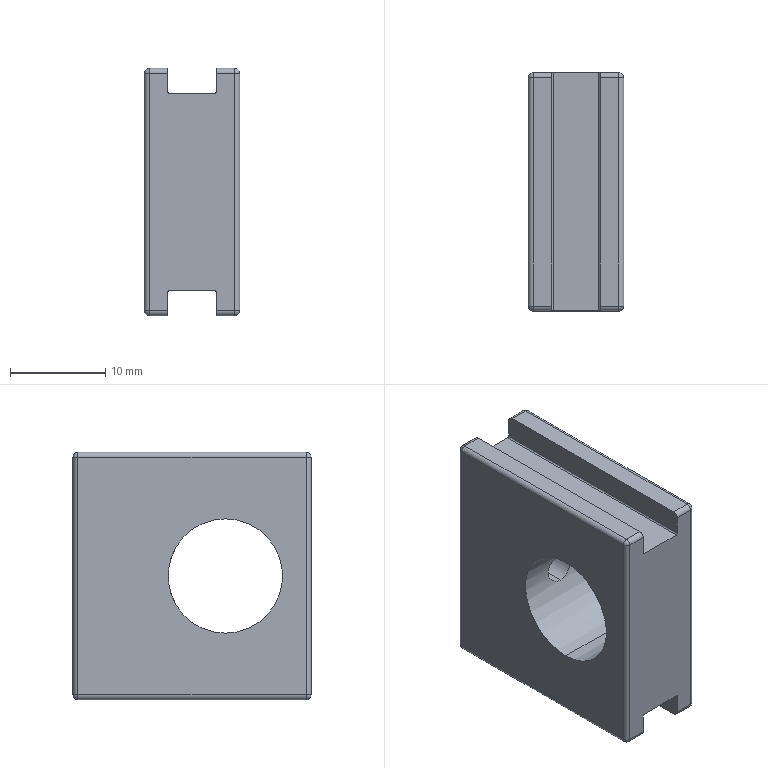Part | NX | features BREP 1 | 1 solid | 46 faces | box 10 x 25 x 25.96 mm | volume 4594 mm3 | cylinder 24 | plane 14 | sphere 8 | commonest cylinder face diameters 1 x16 0.3 x4 3.3 x2 12 x2
STEP:
#1=CARTESIAN_POINT('',(5.,14.769,-10.65));
#2=VERTEX_POINT('',#1);
#3=CARTESIAN_POINT('',(5.,14.769,-7.35));
#4=VERTEX_POINT('',#3);
#5=CARTESIAN_POINT('',(5.,14.769,-7.35));
#6=CARTESIAN_POINT('',(4.795,14.769,-7.35));
#7=CARTESIAN_POINT('',(4.408,14.795,-7.444));
#8=CARTESIAN_POINT('',(4.152,14.83,-7.575));
#9=CARTESIAN_POINT('',(3.816,14.886,-7.821));
#10=CARTESIAN_POINT('',(3.579,14.94,-8.145));
#11=CARTESIAN_POINT('',(3.478,14.966,-8.341));
#12=CARTESIAN_POINT('',(3.365,14.995,-8.693));
#13=CARTESIAN_POINT('',(3.342,15.002,-9.));
#14=CARTESIAN_POINT('',(3.365,14.995,-9.307));
#15=CARTESIAN_POINT('',(3.479,14.966,-9.66));
#16=CARTESIAN_POINT('',(3.58,14.94,-9.856));
#17=CARTESIAN_POINT('',(3.817,14.886,-10.18));
#18=CARTESIAN_POINT('',(4.153,14.83,-10.426));
#19=CARTESIAN_POINT('',(4.41,14.794,-10.557));
#20=CARTESIAN_POINT('',(4.796,14.769,-10.65));
#21=CARTESIAN_POINT('',(5.,14.769,-10.65));
#22=B_SPLINE_CURVE_WITH_KNOTS('',3,(#5,#6,#7,#8,#9,#10,#11,#12,#13,#14,#15,#16,#17,#18,#19,#20,#21),.UNSPECIFIED.,.F.,.F.,(4,1,1,1,1,1,1,1,1,1,1,1,1,1,4),(0.,0.125,0.1875,0.25,0.3125,0.375,0.4375,0.5,0.5625,0.625,0.6875,0.75,0.8125,0.875,1.),.UNSPECIFIED.);
#23=EDGE_CURVE('',#2,#4,#22,.F.);
#24=ORIENTED_EDGE('',*,*,#23,.F.);
#25=CARTESIAN_POINT('',(5.,25.,-10.65));
#26=VERTEX_POINT('',#25);
#27=CARTESIAN_POINT('',(5.,25.,-10.65));
#28=DIRECTION('',(0.,1.,0.));
#29=VECTOR('',#28,1000.);
#30=LINE('',#27,#29);
#31=EDGE_CURVE('',#26,#2,#30,.F.);
#32=ORIENTED_EDGE('',*,*,#31,.F.);
#33=CARTESIAN_POINT('',(5.,25.,-7.35));
#34=VERTEX_POINT('',#33);
#35=CARTESIAN_POINT('',(5.,25.,-9.));
#36=DIRECTION('',(0.,1.,0.));
#37=DIRECTION('',(0.,0.,1.));
#38=AXIS2_PLACEMENT_3D('',#35,#36,#37);
#39=CIRCLE('',#38,1.65);
#40=EDGE_CURVE('',#26,#34,#39,.T.);
#41=ORIENTED_EDGE('',*,*,#40,.T.);
#42=CARTESIAN_POINT('',(5.,25.,-7.35));
#43=DIRECTION('',(0.,1.,0.));
#44=VECTOR('',#43,1000.);
#45=LINE('',#42,#44);
#46=EDGE_CURVE('',#34,#4,#45,.F.);
#47=ORIENTED_EDGE('',*,*,#46,.T.);
#48=EDGE_LOOP('',(#24,#32,#41,#47));
#49=FACE_BOUND('',#48,.T.);
#50=CARTESIAN_POINT('',(5.,25.,-9.));
#51=DIRECTION('',(0.,1.,0.));
#52=DIRECTION('',(0.,0.,1.));
#53=AXIS2_PLACEMENT_3D('',#50,#51,#52);
#54=CYLINDRICAL_SURFACE('',#53,1.65);
#55=ADVANCED_FACE('',(#49),#54,.F.);
#56=CARTESIAN_POINT('',(10.,9.,-15.));
#57=VERTEX_POINT('',#56);
#58=CARTESIAN_POINT('',(10.,9.,-3.));
#59=VERTEX_POINT('',#58);
#60=CARTESIAN_POINT('',(10.,9.,-9.));
#61=DIRECTION('',(-1.,0.,0.));
#62=DIRECTION('',(0.,0.,1.));
#63=AXIS2_PLACEMENT_3D('',#60,#61,#62);
#64=CIRCLE('',#63,6.);
#65=EDGE_CURVE('',#57,#59,#64,.T.);
#66=ORIENTED_EDGE('',*,*,#65,.F.);
#67=CARTESIAN_POINT('',(0.,9.,-15.));
#68=VERTEX_POINT('',#67);
#69=CARTESIAN_POINT('',(10.,9.,-15.));
#70=DIRECTION('',(-1.,0.,0.));
#71=VECTOR('',#70,1000.);
#72=LINE('',#69,#71);
#73=EDGE_CURVE('',#68,#57,#72,.F.);
#74=ORIENTED_EDGE('',*,*,#73,.F.);
#75=CARTESIAN_POINT('',(0.,9.,-3.));
#76=VERTEX_POINT('',#75);
#77=CARTESIAN_POINT('',(0.,9.,-9.));
#78=DIRECTION('',(1.,0.,0.));
#79=DIRECTION('',(0.,0.,1.));
#80=AXIS2_PLACEMENT_3D('',#77,#78,#79);
#81=CIRCLE('',#80,6.);
#82=EDGE_CURVE('',#76,#68,#81,.T.);
#83=ORIENTED_EDGE('',*,*,#82,.F.);
#84=CARTESIAN_POINT('',(10.,9.,-3.));
#85=DIRECTION('',(-1.,0.,0.));
#86=VECTOR('',#85,1000.);
#87=LINE('',#84,#86);
#88=EDGE_CURVE('',#76,#59,#87,.F.);
#89=ORIENTED_EDGE('',*,*,#88,.T.);
#90=EDGE_LOOP('',(#66,#74,#83,#89));
#91=FACE_BOUND('',#90,.T.);
#92=CARTESIAN_POINT('',(10.,9.,-9.));
#93=DIRECTION('',(-1.,0.,0.));
#94=DIRECTION('',(0.,0.,1.));
#95=AXIS2_PLACEMENT_3D('',#92,#93,#94);
#96=CYLINDRICAL_SURFACE('',#95,6.);
#97=ADVANCED_FACE('',(#91),#96,.F.);
#98=CARTESIAN_POINT('',(7.52,0.5,3.98));
#99=VERTEX_POINT('',#98);
#100=CARTESIAN_POINT('',(7.52,24.5,3.98));
#101=VERTEX_POINT('',#100);
#102=CARTESIAN_POINT('',(7.52,0.,3.98));
#103=DIRECTION('',(0.,1.,0.));
#104=VECTOR('',#103,1000.);
#105=LINE('',#102,#104);
#106=EDGE_CURVE('',#99,#101,#105,.T.);
#107=ORIENTED_EDGE('',*,*,#106,.F.);
#108=CARTESIAN_POINT('',(9.5,0.5,3.98));
#109=VERTEX_POINT('',#108);
#110=CARTESIAN_POINT('',(10.,0.5,3.98));
#111=DIRECTION('',(-1.,0.,0.));
#112=VECTOR('',#111,1000.);
#113=LINE('',#110,#112);
#114=EDGE_CURVE('',#109,#99,#113,.T.);
#115=ORIENTED_EDGE('',*,*,#114,.F.);
#116=CARTESIAN_POINT('',(9.5,24.5,3.98));
#117=VERTEX_POINT('',#116);
#118=CARTESIAN_POINT('',(9.5,25.,3.98));
#119=DIRECTION('',(0.,-1.,0.));
#120=VECTOR('',#119,1000.);
#121=LINE('',#118,#120);
#122=EDGE_CURVE('',#117,#109,#121,.T.);
#123=ORIENTED_EDGE('',*,*,#122,.F.);
#124=CARTESIAN_POINT('',(10.,24.5,3.98));
#125=DIRECTION('',(1.,0.,0.));
#126=VECTOR('',#125,1000.);
#127=LINE('',#124,#126);
#128=EDGE_CURVE('',#101,#117,#127,.T.);
#129=ORIENTED_EDGE('',*,*,#128,.F.);
#130=EDGE_LOOP('',(#107,#115,#123,#129));
#131=FACE_BOUND('',#130,.T.);
#132=CARTESIAN_POINT('',(10.,0.,3.98));
#133=DIRECTION('',(0.,0.,-1.));
#134=DIRECTION('',(0.,-1.,0.));
#135=AXIS2_PLACEMENT_3D('',#132,#133,#134);
#136=PLANE('',#135);
#137=ADVANCED_FACE('',(#131),#136,.F.);
#138=ORIENTED_EDGE('',*,*,#114,.T.);
#139=CARTESIAN_POINT('',(7.52,0.,3.48));
#140=VERTEX_POINT('',#139);
#141=CARTESIAN_POINT('',(7.52,0.5,3.48));
#142=DIRECTION('',(1.,0.,0.));
#143=DIRECTION('',(0.,0.,1.));
#144=AXIS2_PLACEMENT_3D('',#141,#142,#143);
#145=CIRCLE('',#144,0.5);
#146=EDGE_CURVE('',#99,#140,#145,.T.);
#147=ORIENTED_EDGE('',*,*,#146,.T.);
#148=CARTESIAN_POINT('',(9.5,0.,3.48));
#149=VERTEX_POINT('',#148);
#150=CARTESIAN_POINT('',(10.,0.,3.48));
#151=DIRECTION('',(1.,0.,0.));
#152=VECTOR('',#151,1000.);
#153=LINE('',#150,#152);
#154=EDGE_CURVE('',#140,#149,#153,.T.);
#155=ORIENTED_EDGE('',*,*,#154,.T.);
#156=CARTESIAN_POINT('',(9.5,0.5,3.48));
#157=DIRECTION('',(-1.,0.,0.));
#158=DIRECTION('',(0.,0.,1.));
#159=AXIS2_PLACEMENT_3D('',#156,#157,#158);
#160=CIRCLE('',#159,0.5);
#161=EDGE_CURVE('',#149,#109,#160,.T.);
#162=ORIENTED_EDGE('',*,*,#161,.T.);
#163=EDGE_LOOP('',(#138,#147,#155,#162));
#164=FACE_BOUND('',#163,.T.);
#165=CARTESIAN_POINT('',(10.,0.5,3.48));
#166=DIRECTION('',(-1.,0.,0.));
#167=DIRECTION('',(0.,0.,1.));
#168=AXIS2_PLACEMENT_3D('',#165,#166,#167);
#169=CYLINDRICAL_SURFACE('',#168,0.5);
#170=ADVANCED_FACE('',(#164),#169,.T.);
#171=CARTESIAN_POINT('',(0.5,0.,3.48));
#172=VERTEX_POINT('',#171);
#173=CARTESIAN_POINT('',(2.48,0.,3.48));
#174=VERTEX_POINT('',#173);
#175=CARTESIAN_POINT('',(10.,0.,3.48));
#176=DIRECTION('',(1.,0.,0.));
#177=VECTOR('',#176,1000.);
#178=LINE('',#175,#177);
#179=EDGE_CURVE('',#172,#174,#178,.T.);
#180=ORIENTED_EDGE('',*,*,#179,.T.);
#181=CARTESIAN_POINT('',(2.48,0.5,3.98));
#182=VERTEX_POINT('',#181);
#183=CARTESIAN_POINT('',(2.48,0.5,3.48));
#184=DIRECTION('',(-1.,0.,0.));
#185=DIRECTION('',(0.,0.,-1.));
#186=AXIS2_PLACEMENT_3D('',#183,#184,#185);
#187=CIRCLE('',#186,0.5);
#188=EDGE_CURVE('',#174,#182,#187,.T.);
#189=ORIENTED_EDGE('',*,*,#188,.T.);
#190=CARTESIAN_POINT('',(0.5,0.5,3.98));
#191=VERTEX_POINT('',#190);
#192=CARTESIAN_POINT('',(10.,0.5,3.98));
#193=DIRECTION('',(-1.,0.,0.));
#194=VECTOR('',#193,1000.);
#195=LINE('',#192,#194);
#196=EDGE_CURVE('',#182,#191,#195,.T.);
#197=ORIENTED_EDGE('',*,*,#196,.T.);
#198=CARTESIAN_POINT('',(0.5,0.5,3.48));
#199=DIRECTION('',(-1.,0.,0.));
#200=DIRECTION('',(0.,0.,-1.));
#201=AXIS2_PLACEMENT_3D('',#198,#199,#200);
#202=CIRCLE('',#201,0.5);
#203=EDGE_CURVE('',#172,#191,#202,.T.);
#204=ORIENTED_EDGE('',*,*,#203,.F.);
#205=EDGE_LOOP('',(#180,#189,#197,#204));
#206=FACE_BOUND('',#205,.T.);
#207=CARTESIAN_POINT('',(10.,0.5,3.48));
#208=DIRECTION('',(-1.,0.,0.));
#209=DIRECTION('',(0.,0.,1.));
#210=AXIS2_PLACEMENT_3D('',#207,#208,#209);
#211=CYLINDRICAL_SURFACE('',#210,0.5);
#212=ADVANCED_FACE('',(#206),#211,.T.);
#213=CARTESIAN_POINT('',(9.5,25.,3.48));
#214=VERTEX_POINT('',#213);
#215=CARTESIAN_POINT('',(7.52,25.,3.48));
#216=VERTEX_POINT('',#215);
#217=CARTESIAN_POINT('',(10.,25.,3.48));
#218=DIRECTION('',(-1.,0.,0.));
#219=VECTOR('',#218,1000.);
#220=LINE('',#217,#219);
#221=EDGE_CURVE('',#214,#216,#220,.T.);
#222=ORIENTED_EDGE('',*,*,#221,.T.);
#223=CARTESIAN_POINT('',(7.52,24.5,3.48));
#224=DIRECTION('',(1.,0.,0.));
#225=DIRECTION('',(0.,0.,1.));
#226=AXIS2_PLACEMENT_3D('',#223,#224,#225);
#227=CIRCLE('',#226,0.5);
#228=EDGE_CURVE('',#216,#101,#227,.T.);
#229=ORIENTED_EDGE('',*,*,#228,.T.);
#230=ORIENTED_EDGE('',*,*,#128,.T.);
#231=CARTESIAN_POINT('',(9.5,24.5,3.48));
#232=DIRECTION('',(-1.,0.,0.));
#233=DIRECTION('',(0.,0.,1.));
#234=AXIS2_PLACEMENT_3D('',#231,#232,#233);
#235=CIRCLE('',#234,0.5);
#236=EDGE_CURVE('',#117,#214,#235,.T.);
#237=ORIENTED_EDGE('',*,*,#236,.T.);
#238=EDGE_LOOP('',(#222,#229,#230,#237));
#239=FACE_BOUND('',#238,.T.);
#240=CARTESIAN_POINT('',(10.,24.5,3.48));
#241=DIRECTION('',(-1.,0.,0.));
#242=DIRECTION('',(0.,0.,1.));
#243=AXIS2_PLACEMENT_3D('',#240,#241,#242);
#244=CYLINDRICAL_SURFACE('',#243,0.5);
#245=ADVANCED_FACE('',(#239),#244,.T.);
#246=CARTESIAN_POINT('',(0.5,24.5,3.98));
#247=VERTEX_POINT('',#246);
#248=CARTESIAN_POINT('',(2.48,24.5,3.98));
#249=VERTEX_POINT('',#248);
#250=CARTESIAN_POINT('',(10.,24.5,3.98));
#251=DIRECTION('',(1.,0.,0.));
#252=VECTOR('',#251,1000.);
#253=LINE('',#250,#252);
#254=EDGE_CURVE('',#247,#249,#253,.T.);
#255=ORIENTED_EDGE('',*,*,#254,.T.);
#256=CARTESIAN_POINT('',(2.48,25.,3.48));
#257=VERTEX_POINT('',#256);
#258=CARTESIAN_POINT('',(2.48,24.5,3.48));
#259=DIRECTION('',(-1.,0.,0.));
#260=DIRECTION('',(0.,0.,-1.));
#261=AXIS2_PLACEMENT_3D('',#258,#259,#260);
#262=CIRCLE('',#261,0.5);
#263=EDGE_CURVE('',#249,#257,#262,.T.);
#264=ORIENTED_EDGE('',*,*,#263,.T.);
#265=CARTESIAN_POINT('',(0.5,25.,3.48));
#266=VERTEX_POINT('',#265);
#267=CARTESIAN_POINT('',(10.,25.,3.48));
#268=DIRECTION('',(-1.,0.,0.));
#269=VECTOR('',#268,1000.);
#270=LINE('',#267,#269);
#271=EDGE_CURVE('',#257,#266,#270,.T.);
#272=ORIENTED_EDGE('',*,*,#271,.T.);
#273=CARTESIAN_POINT('',(0.5,24.5,3.48));
#274=DIRECTION('',(-1.,0.,0.));
#275=DIRECTION('',(0.,0.,-1.));
#276=AXIS2_PLACEMENT_3D('',#273,#274,#275);
#277=CIRCLE('',#276,0.5);
#278=EDGE_CURVE('',#247,#266,#277,.T.);
#279=ORIENTED_EDGE('',*,*,#278,.F.);
#280=EDGE_LOOP('',(#255,#264,#272,#279));
#281=FACE_BOUND('',#280,.T.);
#282=CARTESIAN_POINT('',(10.,24.5,3.48));
#283=DIRECTION('',(-1.,0.,0.));
#284=DIRECTION('',(0.,0.,1.));
#285=AXIS2_PLACEMENT_3D('',#282,#283,#284);
#286=CYLINDRICAL_SURFACE('',#285,0.5);
#287=ADVANCED_FACE('',(#281),#286,.T.);
#288=CARTESIAN_POINT('',(2.48,0.,1.48));
#289=VERTEX_POINT('',#288);
#290=CARTESIAN_POINT('',(2.48,0.,0.));
#291=DIRECTION('',(0.,0.,-1.));
#292=VECTOR('',#291,1000.);
#293=LINE('',#290,#292);
#294=EDGE_CURVE('',#174,#289,#293,.T.);
#295=ORIENTED_EDGE('',*,*,#294,.F.);
#296=ORIENTED_EDGE('',*,*,#179,.F.);
#297=CARTESIAN_POINT('',(0.5,0.,-21.48));
#298=VERTEX_POINT('',#297);
#299=CARTESIAN_POINT('',(0.5,0.,0.));
#300=DIRECTION('',(0.,0.,1.));
#301=VECTOR('',#300,1000.);
#302=LINE('',#299,#301);
#303=EDGE_CURVE('',#298,#172,#302,.T.);
#304=ORIENTED_EDGE('',*,*,#303,.F.);
#305=CARTESIAN_POINT('',(2.48,0.,-21.48));
#306=VERTEX_POINT('',#305);
#307=CARTESIAN_POINT('',(10.,0.,-21.48));
#308=DIRECTION('',(-1.,0.,0.));
#309=VECTOR('',#308,1000.);
#310=LINE('',#307,#309);
#311=EDGE_CURVE('',#306,#298,#310,.T.);
#312=ORIENTED_EDGE('',*,*,#311,.F.);
#313=CARTESIAN_POINT('',(2.48,0.,-19.48));
#314=VERTEX_POINT('',#313);
#315=CARTESIAN_POINT('',(2.48,0.,0.));
#316=DIRECTION('',(0.,0.,1.));
#317=VECTOR('',#316,1000.);
#318=LINE('',#315,#317);
#319=EDGE_CURVE('',#306,#314,#318,.T.);
#320=ORIENTED_EDGE('',*,*,#319,.T.);
#321=CARTESIAN_POINT('',(2.63,0.,-19.33));
#322=VERTEX_POINT('',#321);
#323=CARTESIAN_POINT('',(2.63,0.,-19.48));
#324=DIRECTION('',(0.,1.,0.));
#325=DIRECTION('',(0.,0.,1.));
#326=AXIS2_PLACEMENT_3D('',#323,#324,#325);
#327=CIRCLE('',#326,0.15);
#328=EDGE_CURVE('',#314,#322,#327,.T.);
#329=ORIENTED_EDGE('',*,*,#328,.T.);
#330=CARTESIAN_POINT('',(7.37,0.,-19.33));
#331=VERTEX_POINT('',#330);
#332=CARTESIAN_POINT('',(10.,0.,-19.33));
#333=DIRECTION('',(-1.,0.,0.));
#334=VECTOR('',#333,1000.);
#335=LINE('',#332,#334);
#336=EDGE_CURVE('',#331,#322,#335,.T.);
#337=ORIENTED_EDGE('',*,*,#336,.F.);
#338=CARTESIAN_POINT('',(7.52,0.,-19.48));
#339=VERTEX_POINT('',#338);
#340=CARTESIAN_POINT('',(7.37,0.,-19.48));
#341=DIRECTION('',(0.,1.,0.));
#342=DIRECTION('',(0.,0.,1.));
#343=AXIS2_PLACEMENT_3D('',#340,#341,#342);
#344=CIRCLE('',#343,0.15);
#345=EDGE_CURVE('',#331,#339,#344,.T.);
#346=ORIENTED_EDGE('',*,*,#345,.T.);
#347=CARTESIAN_POINT('',(7.52,0.,-21.48));
#348=VERTEX_POINT('',#347);
#349=CARTESIAN_POINT('',(7.52,0.,0.));
#350=DIRECTION('',(0.,0.,-1.));
#351=VECTOR('',#350,1000.);
#352=LINE('',#349,#351);
#353=EDGE_CURVE('',#339,#348,#352,.T.);
#354=ORIENTED_EDGE('',*,*,#353,.T.);
#355=CARTESIAN_POINT('',(9.5,0.,-21.48));
#356=VERTEX_POINT('',#355);
#357=CARTESIAN_POINT('',(10.,0.,-21.48));
#358=DIRECTION('',(-1.,0.,0.));
#359=VECTOR('',#358,1000.);
#360=LINE('',#357,#359);
#361=EDGE_CURVE('',#356,#348,#360,.T.);
#362=ORIENTED_EDGE('',*,*,#361,.F.);
#363=CARTESIAN_POINT('',(9.5,0.,0.));
#364=DIRECTION('',(0.,0.,-1.));
#365=VECTOR('',#364,1000.);
#366=LINE('',#363,#365);
#367=EDGE_CURVE('',#149,#356,#366,.T.);
#368=ORIENTED_EDGE('',*,*,#367,.F.);
#369=ORIENTED_EDGE('',*,*,#154,.F.);
#370=CARTESIAN_POINT('',(7.52,0.,1.48));
#371=VERTEX_POINT('',#370);
#372=CARTESIAN_POINT('',(7.52,0.,0.));
#373=DIRECTION('',(0.,0.,1.));
#374=VECTOR('',#373,1000.);
#375=LINE('',#372,#374);
#376=EDGE_CURVE('',#371,#140,#375,.T.);
#377=ORIENTED_EDGE('',*,*,#376,.F.);
#378=CARTESIAN_POINT('',(7.37,0.,1.33));
#379=VERTEX_POINT('',#378);
#380=CARTESIAN_POINT('',(7.37,0.,1.48));
#381=DIRECTION('',(0.,1.,0.));
#382=DIRECTION('',(0.,0.,1.));
#383=AXIS2_PLACEMENT_3D('',#380,#381,#382);
#384=CIRCLE('',#383,0.15);
#385=EDGE_CURVE('',#371,#379,#384,.T.);
#386=ORIENTED_EDGE('',*,*,#385,.T.);
#387=CARTESIAN_POINT('',(2.63,0.,1.33));
#388=VERTEX_POINT('',#387);
#389=CARTESIAN_POINT('',(10.,0.,1.33));
#390=DIRECTION('',(1.,0.,0.));
#391=VECTOR('',#390,1000.);
#392=LINE('',#389,#391);
#393=EDGE_CURVE('',#388,#379,#392,.T.);
#394=ORIENTED_EDGE('',*,*,#393,.F.);
#395=CARTESIAN_POINT('',(2.63,0.,1.48));
#396=DIRECTION('',(0.,1.,0.));
#397=DIRECTION('',(0.,0.,1.));
#398=AXIS2_PLACEMENT_3D('',#395,#396,#397);
#399=CIRCLE('',#398,0.15);
#400=EDGE_CURVE('',#388,#289,#399,.T.);
#401=ORIENTED_EDGE('',*,*,#400,.T.);
#402=EDGE_LOOP('',(#295,#296,#304,#312,#320,#329,#337,#346,#354,#362,#368,#369,#377,#386,#394,#401));
#403=FACE_BOUND('',#402,.T.);
#404=CARTESIAN_POINT('',(10.,0.,0.));
#405=DIRECTION('',(0.,1.,0.));
#406=DIRECTION('',(1.,0.,0.));
#407=AXIS2_PLACEMENT_3D('',#404,#405,#406);
#408=PLANE('',#407);
#409=ADVANCED_FACE('',(#403),#408,.F.);
#410=CARTESIAN_POINT('',(2.48,0.,3.98));
#411=DIRECTION('',(0.,-1.,0.));
#412=VECTOR('',#411,1000.);
#413=LINE('',#410,#412);
#414=EDGE_CURVE('',#249,#182,#413,.T.);
#415=ORIENTED_EDGE('',*,*,#414,.F.);
#416=ORIENTED_EDGE('',*,*,#254,.F.);
#417=CARTESIAN_POINT('',(0.5,0.,3.98));
#418=DIRECTION('',(0.,1.,0.));
#419=VECTOR('',#418,1000.);
#420=LINE('',#417,#419);
#421=EDGE_CURVE('',#191,#247,#420,.T.);
#422=ORIENTED_EDGE('',*,*,#421,.F.);
#423=ORIENTED_EDGE('',*,*,#196,.F.);
#424=EDGE_LOOP('',(#415,#416,#422,#423));
#425=FACE_BOUND('',#424,.T.);
#426=CARTESIAN_POINT('',(10.,0.,3.98));
#427=DIRECTION('',(0.,0.,-1.));
#428=DIRECTION('',(0.,-1.,0.));
#429=AXIS2_PLACEMENT_3D('',#426,#427,#428);
#430=PLANE('',#429);
#431=ADVANCED_FACE('',(#425),#430,.F.);
#432=CARTESIAN_POINT('',(7.37,25.,1.33));
#433=VERTEX_POINT('',#432);
#434=CARTESIAN_POINT('',(2.63,25.,1.33));
#435=VERTEX_POINT('',#434);
#436=CARTESIAN_POINT('',(10.,25.,1.33));
#437=DIRECTION('',(-1.,0.,0.));
#438=VECTOR('',#437,1000.);
#439=LINE('',#436,#438);
#440=EDGE_CURVE('',#433,#435,#439,.T.);
#441=ORIENTED_EDGE('',*,*,#440,.F.);
#442=CARTESIAN_POINT('',(7.52,25.,1.48));
#443=VERTEX_POINT('',#442);
#444=CARTESIAN_POINT('',(7.37,25.,1.48));
#445=DIRECTION('',(0.,-1.,0.));
#446=DIRECTION('',(0.,0.,-1.));
#447=AXIS2_PLACEMENT_3D('',#444,#445,#446);
#448=CIRCLE('',#447,0.15);
#449=EDGE_CURVE('',#433,#443,#448,.T.);
#450=ORIENTED_EDGE('',*,*,#449,.T.);
#451=CARTESIAN_POINT('',(7.52,25.,1.016));
#452=DIRECTION('',(0.,0.,1.));
#453=VECTOR('',#452,1000.);
#454=LINE('',#451,#453);
#455=EDGE_CURVE('',#443,#216,#454,.T.);
#456=ORIENTED_EDGE('',*,*,#455,.T.);
#457=ORIENTED_EDGE('',*,*,#221,.F.);
#458=CARTESIAN_POINT('',(9.5,25.,-21.48));
#459=VERTEX_POINT('',#458);
#460=CARTESIAN_POINT('',(9.5,25.,0.));
#461=DIRECTION('',(0.,0.,1.));
#462=VECTOR('',#461,1000.);
#463=LINE('',#460,#462);
#464=EDGE_CURVE('',#459,#214,#463,.T.);
#465=ORIENTED_EDGE('',*,*,#464,.F.);
#466=CARTESIAN_POINT('',(7.52,25.,-21.48));
#467=VERTEX_POINT('',#466);
#468=CARTESIAN_POINT('',(10.,25.,-21.48));
#469=DIRECTION('',(1.,0.,0.));
#470=VECTOR('',#469,1000.);
#471=LINE('',#468,#470);
#472=EDGE_CURVE('',#467,#459,#471,.T.);
#473=ORIENTED_EDGE('',*,*,#472,.F.);
#474=CARTESIAN_POINT('',(7.52,25.,-19.48));
#475=VERTEX_POINT('',#474);
#476=CARTESIAN_POINT('',(7.52,25.,-19.016));
#477=DIRECTION('',(0.,0.,-1.));
#478=VECTOR('',#477,1000.);
#479=LINE('',#476,#478);
#480=EDGE_CURVE('',#475,#467,#479,.T.);
#481=ORIENTED_EDGE('',*,*,#480,.F.);
#482=CARTESIAN_POINT('',(7.37,25.,-19.33));
#483=VERTEX_POINT('',#482);
#484=CARTESIAN_POINT('',(7.37,25.,-19.48));
#485=DIRECTION('',(0.,-1.,0.));
#486=DIRECTION('',(0.,0.,-1.));
#487=AXIS2_PLACEMENT_3D('',#484,#485,#486);
#488=CIRCLE('',#487,0.15);
#489=EDGE_CURVE('',#475,#483,#488,.T.);
#490=ORIENTED_EDGE('',*,*,#489,.T.);
#491=CARTESIAN_POINT('',(2.63,25.,-19.33));
#492=VERTEX_POINT('',#491);
#493=CARTESIAN_POINT('',(10.,25.,-19.33));
#494=DIRECTION('',(1.,0.,0.));
#495=VECTOR('',#494,1000.);
#496=LINE('',#493,#495);
#497=EDGE_CURVE('',#492,#483,#496,.T.);
#498=ORIENTED_EDGE('',*,*,#497,.F.);
#499=CARTESIAN_POINT('',(2.48,25.,-19.48));
#500=VERTEX_POINT('',#499);
#501=CARTESIAN_POINT('',(2.63,25.,-19.48));
#502=DIRECTION('',(0.,-1.,0.));
#503=DIRECTION('',(0.,0.,-1.));
#504=AXIS2_PLACEMENT_3D('',#501,#502,#503);
#505=CIRCLE('',#504,0.15);
#506=EDGE_CURVE('',#492,#500,#505,.T.);
#507=ORIENTED_EDGE('',*,*,#506,.T.);
#508=CARTESIAN_POINT('',(2.48,25.,-21.48));
#509=VERTEX_POINT('',#508);
#510=CARTESIAN_POINT('',(2.48,25.,0.));
#511=DIRECTION('',(0.,0.,-1.));
#512=VECTOR('',#511,1000.);
#513=LINE('',#510,#512);
#514=EDGE_CURVE('',#500,#509,#513,.T.);
#515=ORIENTED_EDGE('',*,*,#514,.T.);
#516=CARTESIAN_POINT('',(0.5,25.,-21.48));
#517=VERTEX_POINT('',#516);
#518=CARTESIAN_POINT('',(10.,25.,-21.48));
#519=DIRECTION('',(1.,0.,0.));
#520=VECTOR('',#519,1000.);
#521=LINE('',#518,#520);
#522=EDGE_CURVE('',#517,#509,#521,.T.);
#523=ORIENTED_EDGE('',*,*,#522,.F.);
#524=CARTESIAN_POINT('',(0.5,25.,0.));
#525=DIRECTION('',(0.,0.,-1.));
#526=VECTOR('',#525,1000.);
#527=LINE('',#524,#526);
#528=EDGE_CURVE('',#266,#517,#527,.T.);
#529=ORIENTED_EDGE('',*,*,#528,.F.);
#530=ORIENTED_EDGE('',*,*,#271,.F.);
#531=CARTESIAN_POINT('',(2.48,25.,1.48));
#532=VERTEX_POINT('',#531);
#533=CARTESIAN_POINT('',(2.48,25.,0.));
#534=DIRECTION('',(0.,0.,1.));
#535=VECTOR('',#534,1000.);
#536=LINE('',#533,#535);
#537=EDGE_CURVE('',#532,#257,#536,.T.);
#538=ORIENTED_EDGE('',*,*,#537,.F.);
#539=CARTESIAN_POINT('',(2.63,25.,1.48));
#540=DIRECTION('',(0.,-1.,0.));
#541=DIRECTION('',(0.,0.,-1.));
#542=AXIS2_PLACEMENT_3D('',#539,#540,#541);
#543=CIRCLE('',#542,0.15);
#544=EDGE_CURVE('',#532,#435,#543,.T.);
#545=ORIENTED_EDGE('',*,*,#544,.T.);
#546=EDGE_LOOP('',(#441,#450,#456,#457,#465,#473,#481,#490,#498,#507,#515,#523,#529,#530,#538,#545));
#547=FACE_BOUND('',#546,.T.);
#548=CARTESIAN_POINT('',(5.,25.,-9.));
#549=DIRECTION('',(0.,1.,0.));
#550=DIRECTION('',(0.,0.,1.));
#551=AXIS2_PLACEMENT_3D('',#548,#549,#550);
#552=CIRCLE('',#551,1.65);
#553=EDGE_CURVE('',#34,#26,#552,.T.);
#554=ORIENTED_EDGE('',*,*,#553,.F.);
#555=ORIENTED_EDGE('',*,*,#40,.F.);
#556=EDGE_LOOP('',(#554,#555));
#557=FACE_BOUND('',#556,.T.);
#558=CARTESIAN_POINT('',(10.,25.,0.));
#559=DIRECTION('',(0.,-1.,0.));
#560=DIRECTION('',(0.,0.,-1.));
#561=AXIS2_PLACEMENT_3D('',#558,#559,#560);
#562=PLANE('',#561);
#563=ADVANCED_FACE('',(#547,#557),#562,.F.);
#564=CARTESIAN_POINT('',(0.,0.5,3.48));
#565=VERTEX_POINT('',#564);
#566=CARTESIAN_POINT('',(0.,24.5,3.48));
#567=VERTEX_POINT('',#566);
#568=CARTESIAN_POINT('',(0.,25.,3.48));
#569=DIRECTION('',(0.,1.,0.));
#570=VECTOR('',#569,1000.);
#571=LINE('',#568,#570);
#572=EDGE_CURVE('',#565,#567,#571,.T.);
#573=ORIENTED_EDGE('',*,*,#572,.T.);
#574=CARTESIAN_POINT('',(0.,24.5,-21.48));
#575=VERTEX_POINT('',#574);
#576=CARTESIAN_POINT('',(0.,24.5,0.));
#577=DIRECTION('',(0.,0.,-1.));
#578=VECTOR('',#577,1000.);
#579=LINE('',#576,#578);
#580=EDGE_CURVE('',#567,#575,#579,.T.);
#581=ORIENTED_EDGE('',*,*,#580,.T.);
#582=CARTESIAN_POINT('',(0.,0.5,-21.48));
#583=VERTEX_POINT('',#582);
#584=CARTESIAN_POINT('',(0.,25.,-21.48));
#585=DIRECTION('',(0.,-1.,0.));
#586=VECTOR('',#585,1000.);
#587=LINE('',#584,#586);
#588=EDGE_CURVE('',#575,#583,#587,.T.);
#589=ORIENTED_EDGE('',*,*,#588,.T.);
#590=CARTESIAN_POINT('',(0.,0.5,0.));
#591=DIRECTION('',(0.,0.,1.));
#592=VECTOR('',#591,1000.);
#593=LINE('',#590,#592);
#594=EDGE_CURVE('',#583,#565,#593,.T.);
#595=ORIENTED_EDGE('',*,*,#594,.T.);
#596=EDGE_LOOP('',(#573,#581,#589,#595));
#597=FACE_BOUND('',#596,.T.);
#598=ORIENTED_EDGE('',*,*,#82,.T.);
#599=CARTESIAN_POINT('',(0.,9.,-9.));
#600=DIRECTION('',(1.,0.,0.));
#601=DIRECTION('',(0.,0.,1.));
#602=AXIS2_PLACEMENT_3D('',#599,#600,#601);
#603=CIRCLE('',#602,6.);
#604=EDGE_CURVE('',#68,#76,#603,.T.);
#605=ORIENTED_EDGE('',*,*,#604,.T.);
#606=EDGE_LOOP('',(#598,#605));
#607=FACE_BOUND('',#606,.T.);
#608=CARTESIAN_POINT('',(0.,25.,0.));
#609=DIRECTION('',(-1.,0.,0.));
#610=DIRECTION('',(0.,0.,1.));
#611=AXIS2_PLACEMENT_3D('',#608,#609,#610);
#612=PLANE('',#611);
#613=ADVANCED_FACE('',(#597,#607),#612,.T.);
#614=ORIENTED_EDGE('',*,*,#73,.T.);
#615=CARTESIAN_POINT('',(10.,9.,-9.));
#616=DIRECTION('',(-1.,0.,0.));
#617=DIRECTION('',(0.,0.,1.));
#618=AXIS2_PLACEMENT_3D('',#615,#616,#617);
#619=CIRCLE('',#618,6.);
#620=EDGE_CURVE('',#59,#57,#619,.T.);
#621=ORIENTED_EDGE('',*,*,#620,.F.);
#622=ORIENTED_EDGE('',*,*,#88,.F.);
#623=ORIENTED_EDGE('',*,*,#604,.F.);
#624=EDGE_LOOP('',(#614,#621,#622,#623));
#625=FACE_BOUND('',#624,.T.);
#626=CARTESIAN_POINT('',(5.,14.769,-7.35));
#627=CARTESIAN_POINT('',(5.439,14.769,-7.35));
#628=CARTESIAN_POINT('',(6.29,14.887,-7.708));
#629=CARTESIAN_POINT('',(6.83,15.057,-8.998));
#630=CARTESIAN_POINT('',(6.289,14.886,-10.294));
#631=CARTESIAN_POINT('',(5.438,14.769,-10.65));
#632=CARTESIAN_POINT('',(5.,14.769,-10.65));
#633=B_SPLINE_CURVE_WITH_KNOTS('',3,(#626,#627,#628,#629,#630,#631,#632),.UNSPECIFIED.,.F.,.F.,(4,1,1,1,4),(0.,0.25,0.5,0.75,1.),.UNSPECIFIED.);
#634=EDGE_CURVE('',#4,#2,#633,.T.);
#635=ORIENTED_EDGE('',*,*,#634,.T.);
#636=ORIENTED_EDGE('',*,*,#23,.T.);
#637=EDGE_LOOP('',(#635,#636));
#638=FACE_BOUND('',#637,.T.);
#639=CARTESIAN_POINT('',(10.,9.,-9.));
#640=DIRECTION('',(-1.,0.,0.));
#641=DIRECTION('',(0.,0.,1.));
#642=AXIS2_PLACEMENT_3D('',#639,#640,#641);
#643=CYLINDRICAL_SURFACE('',#642,6.);
#644=ADVANCED_FACE('',(#625,#638),#643,.F.);
#645=CARTESIAN_POINT('',(0.5,24.5,-21.48));
#646=DIRECTION('',(0.,0.,1.));
#647=DIRECTION('',(-1.,0.,0.));
#648=AXIS2_PLACEMENT_3D('',#645,#646,#647);
#649=CIRCLE('',#648,0.5);
#650=EDGE_CURVE('',#517,#575,#649,.T.);
#651=ORIENTED_EDGE('',*,*,#650,.T.);
#652=ORIENTED_EDGE('',*,*,#580,.F.);
#653=CARTESIAN_POINT('',(0.5,24.5,3.48));
#654=DIRECTION('',(0.,0.,-1.));
#655=DIRECTION('',(-1.,0.,0.));
#656=AXIS2_PLACEMENT_3D('',#653,#654,#655);
#657=CIRCLE('',#656,0.5);
#658=EDGE_CURVE('',#567,#266,#657,.T.);
#659=ORIENTED_EDGE('',*,*,#658,.T.);
#660=ORIENTED_EDGE('',*,*,#528,.T.);
#661=EDGE_LOOP('',(#651,#652,#659,#660));
#662=FACE_BOUND('',#661,.T.);
#663=CARTESIAN_POINT('',(0.5,24.5,0.));
#664=DIRECTION('',(0.,0.,-1.));
#665=DIRECTION('',(-1.,0.,0.));
#666=AXIS2_PLACEMENT_3D('',#663,#664,#665);
#667=CYLINDRICAL_SURFACE('',#666,0.5);
#668=ADVANCED_FACE('',(#662),#667,.T.);
#669=CARTESIAN_POINT('',(0.5,0.5,3.48));
#670=DIRECTION('',(0.,1.,0.));
#671=DIRECTION('',(0.,0.,1.));
#672=AXIS2_PLACEMENT_3D('',#669,#670,#671);
#673=CIRCLE('',#672,0.5);
#674=EDGE_CURVE('',#565,#191,#673,.T.);
#675=ORIENTED_EDGE('',*,*,#674,.T.);
#676=ORIENTED_EDGE('',*,*,#421,.T.);
#677=CARTESIAN_POINT('',(0.5,24.5,3.48));
#678=DIRECTION('',(0.,-1.,0.));
#679=DIRECTION('',(0.,0.,1.));
#680=AXIS2_PLACEMENT_3D('',#677,#678,#679);
#681=CIRCLE('',#680,0.5);
#682=EDGE_CURVE('',#247,#567,#681,.T.);
#683=ORIENTED_EDGE('',*,*,#682,.T.);
#684=ORIENTED_EDGE('',*,*,#572,.F.);
#685=EDGE_LOOP('',(#675,#676,#683,#684));
#686=FACE_BOUND('',#685,.T.);
#687=CARTESIAN_POINT('',(0.5,0.,3.48));
#688=DIRECTION('',(0.,1.,0.));
#689=DIRECTION('',(0.,0.,1.));
#690=AXIS2_PLACEMENT_3D('',#687,#688,#689);
#691=CYLINDRICAL_SURFACE('',#690,0.5);
#692=ADVANCED_FACE('',(#686),#691,.T.);
#693=CARTESIAN_POINT('',(0.5,0.5,-21.48));
#694=DIRECTION('',(0.,0.,1.));
#695=DIRECTION('',(1.,0.,0.));
#696=AXIS2_PLACEMENT_3D('',#693,#694,#695);
#697=CIRCLE('',#696,0.5);
#698=EDGE_CURVE('',#583,#298,#697,.T.);
#699=ORIENTED_EDGE('',*,*,#698,.T.);
#700=ORIENTED_EDGE('',*,*,#303,.T.);
#701=CARTESIAN_POINT('',(0.5,0.5,3.48));
#702=DIRECTION('',(0.,0.,-1.));
#703=DIRECTION('',(1.,0.,0.));
#704=AXIS2_PLACEMENT_3D('',#701,#702,#703);
#705=CIRCLE('',#704,0.5);
#706=EDGE_CURVE('',#172,#565,#705,.T.);
#707=ORIENTED_EDGE('',*,*,#706,.T.);
#708=ORIENTED_EDGE('',*,*,#594,.F.);
#709=EDGE_LOOP('',(#699,#700,#707,#708));
#710=FACE_BOUND('',#709,.T.);
#711=CARTESIAN_POINT('',(0.5,0.5,0.));
#712=DIRECTION('',(0.,0.,1.));
#713=DIRECTION('',(1.,0.,0.));
#714=AXIS2_PLACEMENT_3D('',#711,#712,#713);
#715=CYLINDRICAL_SURFACE('',#714,0.5);
#716=ADVANCED_FACE('',(#710),#715,.T.);
#717=CARTESIAN_POINT('',(0.5,0.5,-21.98));
#718=VERTEX_POINT('',#717);
#719=CARTESIAN_POINT('',(0.5,0.5,-21.48));
#720=DIRECTION('',(0.,1.,0.));
#721=DIRECTION('',(0.,0.,-1.));
#722=AXIS2_PLACEMENT_3D('',#719,#720,#721);
#723=CIRCLE('',#722,0.5);
#724=EDGE_CURVE('',#718,#583,#723,.T.);
#725=ORIENTED_EDGE('',*,*,#724,.T.);
#726=ORIENTED_EDGE('',*,*,#588,.F.);
#727=CARTESIAN_POINT('',(0.5,24.5,-21.98));
#728=VERTEX_POINT('',#727);
#729=CARTESIAN_POINT('',(0.5,24.5,-21.48));
#730=DIRECTION('',(0.,-1.,0.));
#731=DIRECTION('',(0.,0.,-1.));
#732=AXIS2_PLACEMENT_3D('',#729,#730,#731);
#733=CIRCLE('',#732,0.5);
#734=EDGE_CURVE('',#575,#728,#733,.T.);
#735=ORIENTED_EDGE('',*,*,#734,.T.);
#736=CARTESIAN_POINT('',(0.5,0.,-21.98));
#737=DIRECTION('',(0.,-1.,0.));
#738=VECTOR('',#737,1000.);
#739=LINE('',#736,#738);
#740=EDGE_CURVE('',#728,#718,#739,.T.);
#741=ORIENTED_EDGE('',*,*,#740,.T.);
#742=EDGE_LOOP('',(#725,#726,#735,#741));
#743=FACE_BOUND('',#742,.T.);
#744=CARTESIAN_POINT('',(0.5,0.,-21.48));
#745=DIRECTION('',(0.,-1.,0.));
#746=DIRECTION('',(0.,0.,-1.));
#747=AXIS2_PLACEMENT_3D('',#744,#745,#746);
#748=CYLINDRICAL_SURFACE('',#747,0.5);
#749=ADVANCED_FACE('',(#743),#748,.T.);
#750=CARTESIAN_POINT('',(10.,0.5,3.48));
#751=VERTEX_POINT('',#750);
#752=CARTESIAN_POINT('',(10.,24.5,3.48));
#753=VERTEX_POINT('',#752);
#754=CARTESIAN_POINT('',(10.,25.,3.48));
#755=DIRECTION('',(0.,1.,0.));
#756=VECTOR('',#755,1000.);
#757=LINE('',#754,#756);
#758=EDGE_CURVE('',#751,#753,#757,.T.);
#759=ORIENTED_EDGE('',*,*,#758,.F.);
#760=CARTESIAN_POINT('',(10.,0.5,-21.48));
#761=VERTEX_POINT('',#760);
#762=CARTESIAN_POINT('',(10.,0.5,0.));
#763=DIRECTION('',(0.,0.,1.));
#764=VECTOR('',#763,1000.);
#765=LINE('',#762,#764);
#766=EDGE_CURVE('',#761,#751,#765,.T.);
#767=ORIENTED_EDGE('',*,*,#766,.F.);
#768=CARTESIAN_POINT('',(10.,24.5,-21.48));
#769=VERTEX_POINT('',#768);
#770=CARTESIAN_POINT('',(10.,25.,-21.48));
#771=DIRECTION('',(0.,-1.,0.));
#772=VECTOR('',#771,1000.);
#773=LINE('',#770,#772);
#774=EDGE_CURVE('',#769,#761,#773,.T.);
#775=ORIENTED_EDGE('',*,*,#774,.F.);
#776=CARTESIAN_POINT('',(10.,24.5,0.));
#777=DIRECTION('',(0.,0.,-1.));
#778=VECTOR('',#777,1000.);
#779=LINE('',#776,#778);
#780=EDGE_CURVE('',#753,#769,#779,.T.);
#781=ORIENTED_EDGE('',*,*,#780,.F.);
#782=EDGE_LOOP('',(#759,#767,#775,#781));
#783=FACE_BOUND('',#782,.T.);
#784=ORIENTED_EDGE('',*,*,#620,.T.);
#785=ORIENTED_EDGE('',*,*,#65,.T.);
#786=EDGE_LOOP('',(#784,#785));
#787=FACE_BOUND('',#786,.T.);
#788=CARTESIAN_POINT('',(10.,25.,0.));
#789=DIRECTION('',(-1.,0.,0.));
#790=DIRECTION('',(0.,0.,1.));
#791=AXIS2_PLACEMENT_3D('',#788,#789,#790);
#792=PLANE('',#791);
#793=ADVANCED_FACE('',(#783,#787),#792,.F.);
#794=CARTESIAN_POINT('',(0.5,24.5,-21.48));
#795=DIRECTION('',(1.,0.,0.));
#796=DIRECTION('',(0.,0.,1.));
#797=AXIS2_PLACEMENT_3D('',#794,#795,#796);
#798=CIRCLE('',#797,0.5);
#799=EDGE_CURVE('',#728,#517,#798,.T.);
#800=ORIENTED_EDGE('',*,*,#799,.F.);
#801=ORIENTED_EDGE('',*,*,#734,.F.);
#802=ORIENTED_EDGE('',*,*,#650,.F.);
#803=EDGE_LOOP('',(#800,#801,#802));
#804=FACE_BOUND('',#803,.T.);
#805=CARTESIAN_POINT('',(0.5,24.5,-21.48));
#806=DIRECTION('',(1.,0.,0.));
#807=DIRECTION('',(0.,0.,-1.));
#808=AXIS2_PLACEMENT_3D('',#805,#806,#807);
#809=SPHERICAL_SURFACE('',#808,0.5);
#810=ADVANCED_FACE('',(#804),#809,.T.);
#811=ORIENTED_EDGE('',*,*,#658,.F.);
#812=ORIENTED_EDGE('',*,*,#682,.F.);
#813=ORIENTED_EDGE('',*,*,#278,.T.);
#814=EDGE_LOOP('',(#811,#812,#813));
#815=FACE_BOUND('',#814,.T.);
#816=CARTESIAN_POINT('',(0.5,24.5,3.48));
#817=DIRECTION('',(1.,0.,0.));
#818=DIRECTION('',(0.,0.,-1.));
#819=AXIS2_PLACEMENT_3D('',#816,#817,#818);
#820=SPHERICAL_SURFACE('',#819,0.5);
#821=ADVANCED_FACE('',(#815),#820,.T.);
#822=ORIENTED_EDGE('',*,*,#674,.F.);
#823=ORIENTED_EDGE('',*,*,#706,.F.);
#824=ORIENTED_EDGE('',*,*,#203,.T.);
#825=EDGE_LOOP('',(#822,#823,#824));
#826=FACE_BOUND('',#825,.T.);
#827=CARTESIAN_POINT('',(0.5,0.5,3.48));
#828=DIRECTION('',(1.,0.,0.));
#829=DIRECTION('',(0.,0.,-1.));
#830=AXIS2_PLACEMENT_3D('',#827,#828,#829);
#831=SPHERICAL_SURFACE('',#830,0.5);
#832=ADVANCED_FACE('',(#826),#831,.T.);
#833=CARTESIAN_POINT('',(0.5,0.5,-21.48));
#834=DIRECTION('',(-1.,0.,0.));
#835=DIRECTION('',(0.,0.,-1.));
#836=AXIS2_PLACEMENT_3D('',#833,#834,#835);
#837=CIRCLE('',#836,0.5);
#838=EDGE_CURVE('',#718,#298,#837,.T.);
#839=ORIENTED_EDGE('',*,*,#838,.T.);
#840=ORIENTED_EDGE('',*,*,#698,.F.);
#841=ORIENTED_EDGE('',*,*,#724,.F.);
#842=EDGE_LOOP('',(#839,#840,#841));
#843=FACE_BOUND('',#842,.T.);
#844=CARTESIAN_POINT('',(0.5,0.5,-21.48));
#845=DIRECTION('',(1.,0.,0.));
#846=DIRECTION('',(0.,0.,-1.));
#847=AXIS2_PLACEMENT_3D('',#844,#845,#846);
#848=SPHERICAL_SURFACE('',#847,0.5);
#849=ADVANCED_FACE('',(#843),#848,.T.);
#850=CARTESIAN_POINT('',(2.48,24.5,-21.98));
#851=VERTEX_POINT('',#850);
#852=CARTESIAN_POINT('',(10.,24.5,-21.98));
#853=DIRECTION('',(-1.,0.,0.));
#854=VECTOR('',#853,1000.);
#855=LINE('',#852,#854);
#856=EDGE_CURVE('',#851,#728,#855,.T.);
#857=ORIENTED_EDGE('',*,*,#856,.F.);
#858=CARTESIAN_POINT('',(2.48,0.5,-21.98));
#859=VERTEX_POINT('',#858);
#860=CARTESIAN_POINT('',(2.48,0.,-21.98));
#861=DIRECTION('',(0.,-1.,0.));
#862=VECTOR('',#861,1000.);
#863=LINE('',#860,#862);
#864=EDGE_CURVE('',#851,#859,#863,.T.);
#865=ORIENTED_EDGE('',*,*,#864,.T.);
#866=CARTESIAN_POINT('',(10.,0.5,-21.98));
#867=DIRECTION('',(1.,0.,0.));
#868=VECTOR('',#867,1000.);
#869=LINE('',#866,#868);
#870=EDGE_CURVE('',#718,#859,#869,.T.);
#871=ORIENTED_EDGE('',*,*,#870,.F.);
#872=ORIENTED_EDGE('',*,*,#740,.F.);
#873=EDGE_LOOP('',(#857,#865,#871,#872));
#874=FACE_BOUND('',#873,.T.);
#875=CARTESIAN_POINT('',(10.,0.,-21.98));
#876=DIRECTION('',(0.,0.,1.));
#877=DIRECTION('',(1.,0.,0.));
#878=AXIS2_PLACEMENT_3D('',#875,#876,#877);
#879=PLANE('',#878);
#880=ADVANCED_FACE('',(#874),#879,.F.);
#881=CARTESIAN_POINT('',(9.5,24.5,3.48));
#882=DIRECTION('',(0.,0.,-1.));
#883=DIRECTION('',(1.,0.,0.));
#884=AXIS2_PLACEMENT_3D('',#881,#882,#883);
#885=CIRCLE('',#884,0.5);
#886=EDGE_CURVE('',#214,#753,#885,.T.);
#887=ORIENTED_EDGE('',*,*,#886,.T.);
#888=ORIENTED_EDGE('',*,*,#780,.T.);
#889=CARTESIAN_POINT('',(9.5,24.5,-21.48));
#890=DIRECTION('',(0.,0.,1.));
#891=DIRECTION('',(1.,0.,0.));
#892=AXIS2_PLACEMENT_3D('',#889,#890,#891);
#893=CIRCLE('',#892,0.5);
#894=EDGE_CURVE('',#769,#459,#893,.T.);
#895=ORIENTED_EDGE('',*,*,#894,.T.);
#896=ORIENTED_EDGE('',*,*,#464,.T.);
#897=EDGE_LOOP('',(#887,#888,#895,#896));
#898=FACE_BOUND('',#897,.T.);
#899=CARTESIAN_POINT('',(9.5,24.5,0.));
#900=DIRECTION('',(0.,0.,1.));
#901=DIRECTION('',(1.,0.,0.));
#902=AXIS2_PLACEMENT_3D('',#899,#900,#901);
#903=CYLINDRICAL_SURFACE('',#902,0.5);
#904=ADVANCED_FACE('',(#898),#903,.T.);
#905=CARTESIAN_POINT('',(9.5,0.5,3.48));
#906=DIRECTION('',(0.,1.,0.));
#907=DIRECTION('',(0.,0.,-1.));
#908=AXIS2_PLACEMENT_3D('',#905,#906,#907);
#909=CIRCLE('',#908,0.5);
#910=EDGE_CURVE('',#109,#751,#909,.T.);
#911=ORIENTED_EDGE('',*,*,#910,.T.);
#912=ORIENTED_EDGE('',*,*,#758,.T.);
#913=CARTESIAN_POINT('',(9.5,24.5,3.48));
#914=DIRECTION('',(0.,-1.,0.));
#915=DIRECTION('',(0.,0.,-1.));
#916=AXIS2_PLACEMENT_3D('',#913,#914,#915);
#917=CIRCLE('',#916,0.5);
#918=EDGE_CURVE('',#753,#117,#917,.T.);
#919=ORIENTED_EDGE('',*,*,#918,.T.);
#920=ORIENTED_EDGE('',*,*,#122,.T.);
#921=EDGE_LOOP('',(#911,#912,#919,#920));
#922=FACE_BOUND('',#921,.T.);
#923=CARTESIAN_POINT('',(9.5,25.,3.48));
#924=DIRECTION('',(0.,-1.,0.));
#925=DIRECTION('',(0.,0.,-1.));
#926=AXIS2_PLACEMENT_3D('',#923,#924,#925);
#927=CYLINDRICAL_SURFACE('',#926,0.5);
#928=ADVANCED_FACE('',(#922),#927,.T.);
#929=CARTESIAN_POINT('',(9.5,0.5,3.48));
#930=DIRECTION('',(0.,0.,-1.));
#931=DIRECTION('',(-1.,0.,0.));
#932=AXIS2_PLACEMENT_3D('',#929,#930,#931);
#933=CIRCLE('',#932,0.5);
#934=EDGE_CURVE('',#751,#149,#933,.T.);
#935=ORIENTED_EDGE('',*,*,#934,.T.);
#936=ORIENTED_EDGE('',*,*,#367,.T.);
#937=CARTESIAN_POINT('',(9.5,0.5,-21.48));
#938=DIRECTION('',(0.,0.,1.));
#939=DIRECTION('',(-1.,0.,0.));
#940=AXIS2_PLACEMENT_3D('',#937,#938,#939);
#941=CIRCLE('',#940,0.5);
#942=EDGE_CURVE('',#356,#761,#941,.T.);
#943=ORIENTED_EDGE('',*,*,#942,.T.);
#944=ORIENTED_EDGE('',*,*,#766,.T.);
#945=EDGE_LOOP('',(#935,#936,#943,#944));
#946=FACE_BOUND('',#945,.T.);
#947=CARTESIAN_POINT('',(9.5,0.5,0.));
#948=DIRECTION('',(0.,0.,-1.));
#949=DIRECTION('',(-1.,0.,0.));
#950=AXIS2_PLACEMENT_3D('',#947,#948,#949);
#951=CYLINDRICAL_SURFACE('',#950,0.5);
#952=ADVANCED_FACE('',(#946),#951,.T.);
#953=CARTESIAN_POINT('',(9.5,0.5,-21.98));
#954=VERTEX_POINT('',#953);
#955=CARTESIAN_POINT('',(9.5,0.5,-21.48));
#956=DIRECTION('',(0.,1.,0.));
#957=DIRECTION('',(0.,0.,1.));
#958=AXIS2_PLACEMENT_3D('',#955,#956,#957);
#959=CIRCLE('',#958,0.5);
#960=EDGE_CURVE('',#761,#954,#959,.T.);
#961=ORIENTED_EDGE('',*,*,#960,.T.);
#962=CARTESIAN_POINT('',(9.5,24.5,-21.98));
#963=VERTEX_POINT('',#962);
#964=CARTESIAN_POINT('',(9.5,25.,-21.98));
#965=DIRECTION('',(0.,1.,0.));
#966=VECTOR('',#965,1000.);
#967=LINE('',#964,#966);
#968=EDGE_CURVE('',#954,#963,#967,.T.);
#969=ORIENTED_EDGE('',*,*,#968,.T.);
#970=CARTESIAN_POINT('',(9.5,24.5,-21.48));
#971=DIRECTION('',(0.,-1.,0.));
#972=DIRECTION('',(0.,0.,1.));
#973=AXIS2_PLACEMENT_3D('',#970,#971,#972);
#974=CIRCLE('',#973,0.5);
#975=EDGE_CURVE('',#963,#769,#974,.T.);
#976=ORIENTED_EDGE('',*,*,#975,.T.);
#977=ORIENTED_EDGE('',*,*,#774,.T.);
#978=EDGE_LOOP('',(#961,#969,#976,#977));
#979=FACE_BOUND('',#978,.T.);
#980=CARTESIAN_POINT('',(9.5,25.,-21.48));
#981=DIRECTION('',(0.,1.,0.));
#982=DIRECTION('',(0.,0.,1.));
#983=AXIS2_PLACEMENT_3D('',#980,#981,#982);
#984=CYLINDRICAL_SURFACE('',#983,0.5);
#985=ADVANCED_FACE('',(#979),#984,.T.);
#986=ORIENTED_EDGE('',*,*,#440,.T.);
#987=CARTESIAN_POINT('',(2.63,0.,1.33));
#988=DIRECTION('',(0.,-1.,0.));
#989=VECTOR('',#988,1000.);
#990=LINE('',#987,#989);
#991=EDGE_CURVE('',#435,#388,#990,.T.);
#992=ORIENTED_EDGE('',*,*,#991,.T.);
#993=ORIENTED_EDGE('',*,*,#393,.T.);
#994=CARTESIAN_POINT('',(7.37,25.,1.33));
#995=DIRECTION('',(0.,1.,0.));
#996=VECTOR('',#995,1000.);
#997=LINE('',#994,#996);
#998=EDGE_CURVE('',#379,#433,#997,.T.);
#999=ORIENTED_EDGE('',*,*,#998,.T.);
#1000=EDGE_LOOP('',(#986,#992,#993,#999));
#1001=FACE_BOUND('',#1000,.T.);
#1002=CARTESIAN_POINT('',(-11.158,0.,1.33));
#1003=DIRECTION('',(0.,0.,1.));
#1004=DIRECTION('',(1.,0.,0.));
#1005=AXIS2_PLACEMENT_3D('',#1002,#1003,#1004);
#1006=PLANE('',#1005);
#1007=ADVANCED_FACE('',(#1001),#1006,.T.);
#1008=CARTESIAN_POINT('',(7.52,24.5,-21.98));
#1009=VERTEX_POINT('',#1008);
#1010=CARTESIAN_POINT('',(7.52,24.5,-21.48));
#1011=DIRECTION('',(-1.,0.,0.));
#1012=DIRECTION('',(0.,0.,-1.));
#1013=AXIS2_PLACEMENT_3D('',#1010,#1011,#1012);
#1014=CIRCLE('',#1013,0.5);
#1015=EDGE_CURVE('',#467,#1009,#1014,.T.);
#1016=ORIENTED_EDGE('',*,*,#1015,.F.);
#1017=ORIENTED_EDGE('',*,*,#472,.T.);
#1018=CARTESIAN_POINT('',(9.5,24.5,-21.48));
#1019=DIRECTION('',(-1.,0.,0.));
#1020=DIRECTION('',(0.,0.,1.));
#1021=AXIS2_PLACEMENT_3D('',#1018,#1019,#1020);
#1022=CIRCLE('',#1021,0.5);
#1023=EDGE_CURVE('',#459,#963,#1022,.T.);
#1024=ORIENTED_EDGE('',*,*,#1023,.T.);
#1025=CARTESIAN_POINT('',(10.,24.5,-21.98));
#1026=DIRECTION('',(-1.,0.,0.));
#1027=VECTOR('',#1026,1000.);
#1028=LINE('',#1025,#1027);
#1029=EDGE_CURVE('',#963,#1009,#1028,.T.);
#1030=ORIENTED_EDGE('',*,*,#1029,.T.);
#1031=EDGE_LOOP('',(#1016,#1017,#1024,#1030));
#1032=FACE_BOUND('',#1031,.T.);
#1033=CARTESIAN_POINT('',(10.,24.5,-21.48));
#1034=DIRECTION('',(-1.,0.,0.));
#1035=DIRECTION('',(0.,0.,1.));
#1036=AXIS2_PLACEMENT_3D('',#1033,#1034,#1035);
#1037=CYLINDRICAL_SURFACE('',#1036,0.5);
#1038=ADVANCED_FACE('',(#1032),#1037,.T.);
#1039=ORIENTED_EDGE('',*,*,#336,.T.);
#1040=CARTESIAN_POINT('',(2.63,25.,-19.33));
#1041=DIRECTION('',(0.,1.,0.));
#1042=VECTOR('',#1041,1000.);
#1043=LINE('',#1040,#1042);
#1044=EDGE_CURVE('',#322,#492,#1043,.T.);
#1045=ORIENTED_EDGE('',*,*,#1044,.T.);
#1046=ORIENTED_EDGE('',*,*,#497,.T.);
#1047=CARTESIAN_POINT('',(7.37,0.,-19.33));
#1048=DIRECTION('',(0.,-1.,0.));
#1049=VECTOR('',#1048,1000.);
#1050=LINE('',#1047,#1049);
#1051=EDGE_CURVE('',#483,#331,#1050,.T.);
#1052=ORIENTED_EDGE('',*,*,#1051,.T.);
#1053=EDGE_LOOP('',(#1039,#1045,#1046,#1052));
#1054=FACE_BOUND('',#1053,.T.);
#1055=CARTESIAN_POINT('',(-11.158,0.,-19.33));
#1056=DIRECTION('',(0.,0.,1.));
#1057=DIRECTION('',(1.,0.,0.));
#1058=AXIS2_PLACEMENT_3D('',#1055,#1056,#1057);
#1059=PLANE('',#1058);
#1060=ADVANCED_FACE('',(#1054),#1059,.F.);
#1061=CARTESIAN_POINT('',(2.48,24.5,-21.48));
#1062=DIRECTION('',(1.,0.,0.));
#1063=DIRECTION('',(0.,0.,1.));
#1064=AXIS2_PLACEMENT_3D('',#1061,#1062,#1063);
#1065=CIRCLE('',#1064,0.5);
#1066=EDGE_CURVE('',#851,#509,#1065,.T.);
#1067=ORIENTED_EDGE('',*,*,#1066,.F.);
#1068=ORIENTED_EDGE('',*,*,#856,.T.);
#1069=ORIENTED_EDGE('',*,*,#799,.T.);
#1070=ORIENTED_EDGE('',*,*,#522,.T.);
#1071=EDGE_LOOP('',(#1067,#1068,#1069,#1070));
#1072=FACE_BOUND('',#1071,.T.);
#1073=CARTESIAN_POINT('',(10.,24.5,-21.48));
#1074=DIRECTION('',(-1.,0.,0.));
#1075=DIRECTION('',(0.,0.,1.));
#1076=AXIS2_PLACEMENT_3D('',#1073,#1074,#1075);
#1077=CYLINDRICAL_SURFACE('',#1076,0.5);
#1078=ADVANCED_FACE('',(#1072),#1077,.T.);
#1079=CARTESIAN_POINT('',(2.48,0.5,-21.48));
#1080=DIRECTION('',(1.,0.,0.));
#1081=DIRECTION('',(0.,0.,1.));
#1082=AXIS2_PLACEMENT_3D('',#1079,#1080,#1081);
#1083=CIRCLE('',#1082,0.5);
#1084=EDGE_CURVE('',#306,#859,#1083,.T.);
#1085=ORIENTED_EDGE('',*,*,#1084,.F.);
#1086=ORIENTED_EDGE('',*,*,#311,.T.);
#1087=ORIENTED_EDGE('',*,*,#838,.F.);
#1088=ORIENTED_EDGE('',*,*,#870,.T.);
#1089=EDGE_LOOP('',(#1085,#1086,#1087,#1088));
#1090=FACE_BOUND('',#1089,.T.);
#1091=CARTESIAN_POINT('',(10.,0.5,-21.48));
#1092=DIRECTION('',(-1.,0.,0.));
#1093=DIRECTION('',(0.,0.,1.));
#1094=AXIS2_PLACEMENT_3D('',#1091,#1092,#1093);
#1095=CYLINDRICAL_SURFACE('',#1094,0.5);
#1096=ADVANCED_FACE('',(#1090),#1095,.T.);
#1097=CARTESIAN_POINT('',(7.52,0.5,-21.98));
#1098=VERTEX_POINT('',#1097);
#1099=CARTESIAN_POINT('',(7.52,0.5,-21.48));
#1100=DIRECTION('',(-1.,0.,0.));
#1101=DIRECTION('',(0.,0.,-1.));
#1102=AXIS2_PLACEMENT_3D('',#1099,#1100,#1101);
#1103=CIRCLE('',#1102,0.5);
#1104=EDGE_CURVE('',#1098,#348,#1103,.T.);
#1105=ORIENTED_EDGE('',*,*,#1104,.F.);
#1106=CARTESIAN_POINT('',(10.,0.5,-21.98));
#1107=DIRECTION('',(1.,0.,0.));
#1108=VECTOR('',#1107,1000.);
#1109=LINE('',#1106,#1108);
#1110=EDGE_CURVE('',#1098,#954,#1109,.T.);
#1111=ORIENTED_EDGE('',*,*,#1110,.T.);
#1112=CARTESIAN_POINT('',(9.5,0.5,-21.48));
#1113=DIRECTION('',(-1.,0.,0.));
#1114=DIRECTION('',(0.,0.,1.));
#1115=AXIS2_PLACEMENT_3D('',#1112,#1113,#1114);
#1116=CIRCLE('',#1115,0.5);
#1117=EDGE_CURVE('',#954,#356,#1116,.T.);
#1118=ORIENTED_EDGE('',*,*,#1117,.T.);
#1119=ORIENTED_EDGE('',*,*,#361,.T.);
#1120=EDGE_LOOP('',(#1105,#1111,#1118,#1119));
#1121=FACE_BOUND('',#1120,.T.);
#1122=CARTESIAN_POINT('',(10.,0.5,-21.48));
#1123=DIRECTION('',(-1.,0.,0.));
#1124=DIRECTION('',(0.,0.,1.));
#1125=AXIS2_PLACEMENT_3D('',#1122,#1123,#1124);
#1126=CYLINDRICAL_SURFACE('',#1125,0.5);
#1127=ADVANCED_FACE('',(#1121),#1126,.T.);
#1128=ORIENTED_EDGE('',*,*,#236,.F.);
#1129=ORIENTED_EDGE('',*,*,#918,.F.);
#1130=ORIENTED_EDGE('',*,*,#886,.F.);
#1131=EDGE_LOOP('',(#1128,#1129,#1130));
#1132=FACE_BOUND('',#1131,.T.);
#1133=CARTESIAN_POINT('',(9.5,24.5,3.48));
#1134=DIRECTION('',(1.,0.,0.));
#1135=DIRECTION('',(0.,0.,-1.));
#1136=AXIS2_PLACEMENT_3D('',#1133,#1134,#1135);
#1137=SPHERICAL_SURFACE('',#1136,0.5);
#1138=ADVANCED_FACE('',(#1132),#1137,.T.);
#1139=ORIENTED_EDGE('',*,*,#1023,.F.);
#1140=ORIENTED_EDGE('',*,*,#894,.F.);
#1141=ORIENTED_EDGE('',*,*,#975,.F.);
#1142=EDGE_LOOP('',(#1139,#1140,#1141));
#1143=FACE_BOUND('',#1142,.T.);
#1144=CARTESIAN_POINT('',(9.5,24.5,-21.48));
#1145=DIRECTION('',(1.,0.,0.));
#1146=DIRECTION('',(0.,0.,-1.));
#1147=AXIS2_PLACEMENT_3D('',#1144,#1145,#1146);
#1148=SPHERICAL_SURFACE('',#1147,0.5);
#1149=ADVANCED_FACE('',(#1143),#1148,.T.);
#1150=ORIENTED_EDGE('',*,*,#910,.F.);
#1151=ORIENTED_EDGE('',*,*,#161,.F.);
#1152=ORIENTED_EDGE('',*,*,#934,.F.);
#1153=EDGE_LOOP('',(#1150,#1151,#1152));
#1154=FACE_BOUND('',#1153,.T.);
#1155=CARTESIAN_POINT('',(9.5,0.5,3.48));
#1156=DIRECTION('',(1.,0.,0.));
#1157=DIRECTION('',(0.,0.,-1.));
#1158=AXIS2_PLACEMENT_3D('',#1155,#1156,#1157);
#1159=SPHERICAL_SURFACE('',#1158,0.5);
#1160=ADVANCED_FACE('',(#1154),#1159,.T.);
#1161=ORIENTED_EDGE('',*,*,#960,.F.);
#1162=ORIENTED_EDGE('',*,*,#942,.F.);
#1163=ORIENTED_EDGE('',*,*,#1117,.F.);
#1164=EDGE_LOOP('',(#1161,#1162,#1163));
#1165=FACE_BOUND('',#1164,.T.);
#1166=CARTESIAN_POINT('',(9.5,0.5,-21.48));
#1167=DIRECTION('',(1.,0.,0.));
#1168=DIRECTION('',(0.,0.,-1.));
#1169=AXIS2_PLACEMENT_3D('',#1166,#1167,#1168);
#1170=SPHERICAL_SURFACE('',#1169,0.5);
#1171=ADVANCED_FACE('',(#1165),#1170,.T.);
#1172=ORIENTED_EDGE('',*,*,#1110,.F.);
#1173=CARTESIAN_POINT('',(7.52,0.,-21.98));
#1174=DIRECTION('',(0.,1.,0.));
#1175=VECTOR('',#1174,1000.);
#1176=LINE('',#1173,#1175);
#1177=EDGE_CURVE('',#1098,#1009,#1176,.T.);
#1178=ORIENTED_EDGE('',*,*,#1177,.T.);
#1179=ORIENTED_EDGE('',*,*,#1029,.F.);
#1180=ORIENTED_EDGE('',*,*,#968,.F.);
#1181=EDGE_LOOP('',(#1172,#1178,#1179,#1180));
#1182=FACE_BOUND('',#1181,.T.);
#1183=CARTESIAN_POINT('',(10.,0.,-21.98));
#1184=DIRECTION('',(0.,0.,1.));
#1185=DIRECTION('',(1.,0.,0.));
#1186=AXIS2_PLACEMENT_3D('',#1183,#1184,#1185);
#1187=PLANE('',#1186);
#1188=ADVANCED_FACE('',(#1182),#1187,.F.);
#1189=ORIENTED_EDGE('',*,*,#31,.T.);
#1190=ORIENTED_EDGE('',*,*,#634,.F.);
#1191=ORIENTED_EDGE('',*,*,#46,.F.);
#1192=ORIENTED_EDGE('',*,*,#553,.T.);
#1193=EDGE_LOOP('',(#1189,#1190,#1191,#1192));
#1194=FACE_BOUND('',#1193,.T.);
#1195=CARTESIAN_POINT('',(5.,25.,-9.));
#1196=DIRECTION('',(0.,1.,0.));
#1197=DIRECTION('',(0.,0.,1.));
#1198=AXIS2_PLACEMENT_3D('',#1195,#1196,#1197);
#1199=CYLINDRICAL_SURFACE('',#1198,1.65);
#1200=ADVANCED_FACE('',(#1194),#1199,.F.);
#1201=ORIENTED_EDGE('',*,*,#514,.F.);
#1202=CARTESIAN_POINT('',(2.48,0.,-19.48));
#1203=DIRECTION('',(0.,-1.,0.));
#1204=VECTOR('',#1203,1000.);
#1205=LINE('',#1202,#1204);
#1206=EDGE_CURVE('',#500,#314,#1205,.T.);
#1207=ORIENTED_EDGE('',*,*,#1206,.T.);
#1208=ORIENTED_EDGE('',*,*,#319,.F.);
#1209=ORIENTED_EDGE('',*,*,#1084,.T.);
#1210=ORIENTED_EDGE('',*,*,#864,.F.);
#1211=ORIENTED_EDGE('',*,*,#1066,.T.);
#1212=EDGE_LOOP('',(#1201,#1207,#1208,#1209,#1210,#1211));
#1213=FACE_BOUND('',#1212,.T.);
#1214=CARTESIAN_POINT('',(2.48,-0.0001031,-19.016));
#1215=DIRECTION('',(-1.,0.,0.));
#1216=DIRECTION('',(0.,1.,0.));
#1217=AXIS2_PLACEMENT_3D('',#1214,#1215,#1216);
#1218=PLANE('',#1217);
#1219=ADVANCED_FACE('',(#1213),#1218,.F.);
#1220=ORIENTED_EDGE('',*,*,#353,.F.);
#1221=CARTESIAN_POINT('',(7.52,25.,-19.48));
#1222=DIRECTION('',(0.,1.,0.));
#1223=VECTOR('',#1222,1000.);
#1224=LINE('',#1221,#1223);
#1225=EDGE_CURVE('',#339,#475,#1224,.T.);
#1226=ORIENTED_EDGE('',*,*,#1225,.T.);
#1227=ORIENTED_EDGE('',*,*,#480,.T.);
#1228=ORIENTED_EDGE('',*,*,#1015,.T.);
#1229=ORIENTED_EDGE('',*,*,#1177,.F.);
#1230=ORIENTED_EDGE('',*,*,#1104,.T.);
#1231=EDGE_LOOP('',(#1220,#1226,#1227,#1228,#1229,#1230));
#1232=FACE_BOUND('',#1231,.T.);
#1233=CARTESIAN_POINT('',(7.52,-0.0001031,-19.016));
#1234=DIRECTION('',(1.,0.,0.));
#1235=DIRECTION('',(0.,0.,-1.));
#1236=AXIS2_PLACEMENT_3D('',#1233,#1234,#1235);
#1237=PLANE('',#1236);
#1238=ADVANCED_FACE('',(#1232),#1237,.F.);
#1239=ORIENTED_EDGE('',*,*,#294,.T.);
#1240=CARTESIAN_POINT('',(2.48,25.,1.48));
#1241=DIRECTION('',(0.,1.,0.));
#1242=VECTOR('',#1241,1000.);
#1243=LINE('',#1240,#1242);
#1244=EDGE_CURVE('',#289,#532,#1243,.T.);
#1245=ORIENTED_EDGE('',*,*,#1244,.T.);
#1246=ORIENTED_EDGE('',*,*,#537,.T.);
#1247=ORIENTED_EDGE('',*,*,#263,.F.);
#1248=ORIENTED_EDGE('',*,*,#414,.T.);
#1249=ORIENTED_EDGE('',*,*,#188,.F.);
#1250=EDGE_LOOP('',(#1239,#1245,#1246,#1247,#1248,#1249));
#1251=FACE_BOUND('',#1250,.T.);
#1252=CARTESIAN_POINT('',(2.48,-0.0001031,1.016));
#1253=DIRECTION('',(1.,0.,0.));
#1254=DIRECTION('',(0.,0.,1.));
#1255=AXIS2_PLACEMENT_3D('',#1252,#1253,#1254);
#1256=PLANE('',#1255);
#1257=ADVANCED_FACE('',(#1251),#1256,.T.);
#1258=ORIENTED_EDGE('',*,*,#455,.F.);
#1259=CARTESIAN_POINT('',(7.52,0.,1.48));
#1260=DIRECTION('',(0.,-1.,0.));
#1261=VECTOR('',#1260,1000.);
#1262=LINE('',#1259,#1261);
#1263=EDGE_CURVE('',#443,#371,#1262,.T.);
#1264=ORIENTED_EDGE('',*,*,#1263,.T.);
#1265=ORIENTED_EDGE('',*,*,#376,.T.);
#1266=ORIENTED_EDGE('',*,*,#146,.F.);
#1267=ORIENTED_EDGE('',*,*,#106,.T.);
#1268=ORIENTED_EDGE('',*,*,#228,.F.);
#1269=EDGE_LOOP('',(#1258,#1264,#1265,#1266,#1267,#1268));
#1270=FACE_BOUND('',#1269,.T.);
#1271=CARTESIAN_POINT('',(7.52,-0.0001031,1.016));
#1272=DIRECTION('',(-1.,0.,0.));
#1273=DIRECTION('',(0.,0.,1.));
#1274=AXIS2_PLACEMENT_3D('',#1271,#1272,#1273);
#1275=PLANE('',#1274);
#1276=ADVANCED_FACE('',(#1270),#1275,.T.);
#1277=ORIENTED_EDGE('',*,*,#400,.F.);
#1278=ORIENTED_EDGE('',*,*,#991,.F.);
#1279=ORIENTED_EDGE('',*,*,#544,.F.);
#1280=ORIENTED_EDGE('',*,*,#1244,.F.);
#1281=EDGE_LOOP('',(#1277,#1278,#1279,#1280));
#1282=FACE_BOUND('',#1281,.T.);
#1283=CARTESIAN_POINT('',(2.63,-0.0001031,1.48));
#1284=DIRECTION('',(0.,-1.,0.));
#1285=DIRECTION('',(0.,0.,-1.));
#1286=AXIS2_PLACEMENT_3D('',#1283,#1284,#1285);
#1287=CYLINDRICAL_SURFACE('',#1286,0.15);
#1288=ADVANCED_FACE('',(#1282),#1287,.F.);
#1289=ORIENTED_EDGE('',*,*,#328,.F.);
#1290=ORIENTED_EDGE('',*,*,#1206,.F.);
#1291=ORIENTED_EDGE('',*,*,#506,.F.);
#1292=ORIENTED_EDGE('',*,*,#1044,.F.);
#1293=EDGE_LOOP('',(#1289,#1290,#1291,#1292));
#1294=FACE_BOUND('',#1293,.T.);
#1295=CARTESIAN_POINT('',(2.63,0.,-19.48));
#1296=DIRECTION('',(0.,-1.,0.));
#1297=DIRECTION('',(0.,0.,-1.));
#1298=AXIS2_PLACEMENT_3D('',#1295,#1296,#1297);
#1299=CYLINDRICAL_SURFACE('',#1298,0.15);
#1300=ADVANCED_FACE('',(#1294),#1299,.F.);
#1301=ORIENTED_EDGE('',*,*,#385,.F.);
#1302=ORIENTED_EDGE('',*,*,#1263,.F.);
#1303=ORIENTED_EDGE('',*,*,#449,.F.);
#1304=ORIENTED_EDGE('',*,*,#998,.F.);
#1305=EDGE_LOOP('',(#1301,#1302,#1303,#1304));
#1306=FACE_BOUND('',#1305,.T.);
#1307=CARTESIAN_POINT('',(7.37,0.,1.48));
#1308=DIRECTION('',(0.,-1.,0.));
#1309=DIRECTION('',(0.,0.,-1.));
#1310=AXIS2_PLACEMENT_3D('',#1307,#1308,#1309);
#1311=CYLINDRICAL_SURFACE('',#1310,0.15);
#1312=ADVANCED_FACE('',(#1306),#1311,.F.);
#1313=ORIENTED_EDGE('',*,*,#345,.F.);
#1314=ORIENTED_EDGE('',*,*,#1051,.F.);
#1315=ORIENTED_EDGE('',*,*,#489,.F.);
#1316=ORIENTED_EDGE('',*,*,#1225,.F.);
#1317=EDGE_LOOP('',(#1313,#1314,#1315,#1316));
#1318=FACE_BOUND('',#1317,.T.);
#1319=CARTESIAN_POINT('',(7.37,-0.0001031,-19.48));
#1320=DIRECTION('',(0.,-1.,0.));
#1321=DIRECTION('',(0.,0.,-1.));
#1322=AXIS2_PLACEMENT_3D('',#1319,#1320,#1321);
#1323=CYLINDRICAL_SURFACE('',#1322,0.15);
#1324=ADVANCED_FACE('',(#1318),#1323,.F.);
#1325=CLOSED_SHELL('',(#55,#97,#137,#170,#212,#245,#287,#409,#431,#563,#613,#644,#668,#692,#716,#749,#793,#810,#821,#832,#849,#880,#904,#928,#952,#985,#1007,#1038,#1060,#1078,#1096,#1127,#1138,#1149,#1160,#1171,#1188,#1200,#1219,#1238,#1257,#1276,#1288,#1300,#1312,#1324));
#1326=MANIFOLD_SOLID_BREP('',#1325);
#1327=(LENGTH_UNIT()NAMED_UNIT(*)SI_UNIT(.MILLI.,.METRE.));
#1328=UNCERTAINTY_MEASURE_WITH_UNIT(LENGTH_MEASURE(0.0508),#1327,'','');
#1329=(NAMED_UNIT(*)PLANE_ANGLE_UNIT()SI_UNIT($,.RADIAN.));
#1330=(NAMED_UNIT(*)SI_UNIT($,.STERADIAN.)SOLID_ANGLE_UNIT());
#1331=(GEOMETRIC_REPRESENTATION_CONTEXT(3)GLOBAL_UNCERTAINTY_ASSIGNED_CONTEXT((#1328))GLOBAL_UNIT_ASSIGNED_CONTEXT((#1327,#1329,#1330))REPRESENTATION_CONTEXT('',''));
#1332=ADVANCED_BREP_SHAPE_REPRESENTATION('',(#1326),#1331);